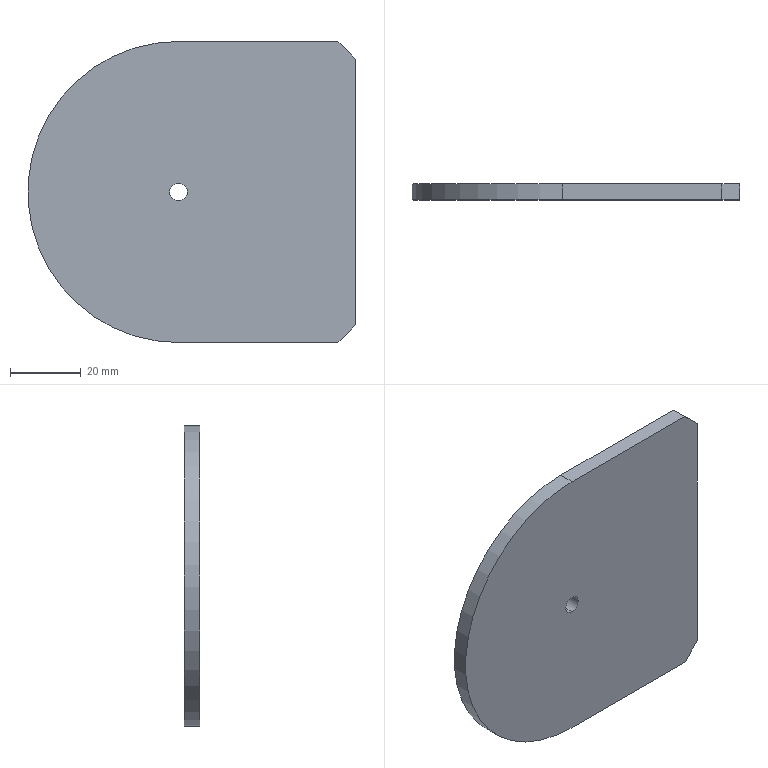Part | SolidWorks | features FlatPattern 1, SMBaseFlange 1, SheetMetal 1 | 1 solid | 10 faces | box 92.5 x 4.5 x 85 mm | volume 31692 mm3 | plane 7 | cylinder 3 | commonest cylinder face diameters 5 x2 85 x1
STEP:
#1=CARTESIAN_POINT('',(0.,-4.5,-2.5));
#2=VERTEX_POINT('',#1);
#3=CARTESIAN_POINT('',(0.,-4.5,2.5));
#4=VERTEX_POINT('',#3);
#5=CARTESIAN_POINT('',(0.,-4.5,0.));
#6=DIRECTION('',(0.,1.,0.));
#7=DIRECTION('',(0.,0.,1.));
#8=AXIS2_PLACEMENT_3D('',#5,#6,#7);
#9=CIRCLE('',#8,2.5);
#10=EDGE_CURVE('',#2,#4,#9,.T.);
#11=ORIENTED_EDGE('',*,*,#10,.F.);
#12=CARTESIAN_POINT('',(0.,0.,-2.5));
#13=VERTEX_POINT('',#12);
#14=CARTESIAN_POINT('',(0.,-4.5,-2.5));
#15=DIRECTION('',(0.,1.,0.));
#16=VECTOR('',#15,1000.);
#17=LINE('',#14,#16);
#18=EDGE_CURVE('',#2,#13,#17,.T.);
#19=ORIENTED_EDGE('',*,*,#18,.T.);
#20=CARTESIAN_POINT('',(0.,0.,2.5));
#21=VERTEX_POINT('',#20);
#22=CARTESIAN_POINT('',(0.,0.,0.));
#23=DIRECTION('',(0.,1.,0.));
#24=DIRECTION('',(0.,0.,1.));
#25=AXIS2_PLACEMENT_3D('',#22,#23,#24);
#26=CIRCLE('',#25,2.5);
#27=EDGE_CURVE('',#13,#21,#26,.T.);
#28=ORIENTED_EDGE('',*,*,#27,.T.);
#29=CARTESIAN_POINT('',(0.,-4.5,2.5));
#30=DIRECTION('',(0.,1.,0.));
#31=VECTOR('',#30,1000.);
#32=LINE('',#29,#31);
#33=EDGE_CURVE('',#4,#21,#32,.T.);
#34=ORIENTED_EDGE('',*,*,#33,.F.);
#35=EDGE_LOOP('',(#11,#19,#28,#34));
#36=FACE_OUTER_BOUND('',#35,.T.);
#37=CARTESIAN_POINT('',(0.,-4.5,0.));
#38=DIRECTION('',(0.,1.,0.));
#39=DIRECTION('',(0.,0.,1.));
#40=AXIS2_PLACEMENT_3D('',#37,#38,#39);
#41=CYLINDRICAL_SURFACE('',#40,2.5);
#42=ADVANCED_FACE('',(#36),#41,.F.);
#43=CARTESIAN_POINT('',(45.,0.,42.5));
#44=VERTEX_POINT('',#43);
#45=CARTESIAN_POINT('',(50.,0.,37.5));
#46=VERTEX_POINT('',#45);
#47=CARTESIAN_POINT('',(45.,0.,42.5));
#48=DIRECTION('',(0.7071,0.,-0.7071));
#49=VECTOR('',#48,1000.);
#50=LINE('',#47,#49);
#51=EDGE_CURVE('',#44,#46,#50,.T.);
#52=ORIENTED_EDGE('',*,*,#51,.F.);
#53=CARTESIAN_POINT('',(45.,-4.5,42.5));
#54=VERTEX_POINT('',#53);
#55=CARTESIAN_POINT('',(45.,-4.5,42.5));
#56=DIRECTION('',(0.,1.,0.));
#57=VECTOR('',#56,1000.);
#58=LINE('',#55,#57);
#59=EDGE_CURVE('',#54,#44,#58,.T.);
#60=ORIENTED_EDGE('',*,*,#59,.F.);
#61=CARTESIAN_POINT('',(50.,-4.5,37.5));
#62=VERTEX_POINT('',#61);
#63=CARTESIAN_POINT('',(45.,-4.5,42.5));
#64=DIRECTION('',(0.7071,0.,-0.7071));
#65=VECTOR('',#64,1000.);
#66=LINE('',#63,#65);
#67=EDGE_CURVE('',#54,#62,#66,.T.);
#68=ORIENTED_EDGE('',*,*,#67,.T.);
#69=CARTESIAN_POINT('',(50.,-4.5,37.5));
#70=DIRECTION('',(0.,1.,0.));
#71=VECTOR('',#70,1000.);
#72=LINE('',#69,#71);
#73=EDGE_CURVE('',#62,#46,#72,.T.);
#74=ORIENTED_EDGE('',*,*,#73,.T.);
#75=EDGE_LOOP('',(#52,#60,#68,#74));
#76=FACE_OUTER_BOUND('',#75,.T.);
#77=CARTESIAN_POINT('',(45.,-4.5,42.5));
#78=DIRECTION('',(0.7071,0.,0.7071));
#79=DIRECTION('',(0.7071,0.,-0.7071));
#80=AXIS2_PLACEMENT_3D('',#77,#78,#79);
#81=PLANE('',#80);
#82=ADVANCED_FACE('',(#76),#81,.T.);
#83=CARTESIAN_POINT('',(0.,0.,42.5));
#84=VERTEX_POINT('',#83);
#85=CARTESIAN_POINT('',(0.,0.,42.5));
#86=DIRECTION('',(1.,0.,0.));
#87=VECTOR('',#86,1000.);
#88=LINE('',#85,#87);
#89=EDGE_CURVE('',#84,#44,#88,.T.);
#90=ORIENTED_EDGE('',*,*,#89,.F.);
#91=CARTESIAN_POINT('',(0.,-4.5,42.5));
#92=VERTEX_POINT('',#91);
#93=CARTESIAN_POINT('',(0.,-4.5,42.5));
#94=DIRECTION('',(0.,1.,0.));
#95=VECTOR('',#94,1000.);
#96=LINE('',#93,#95);
#97=EDGE_CURVE('',#92,#84,#96,.T.);
#98=ORIENTED_EDGE('',*,*,#97,.F.);
#99=CARTESIAN_POINT('',(0.,-4.5,42.5));
#100=DIRECTION('',(1.,0.,0.));
#101=VECTOR('',#100,1000.);
#102=LINE('',#99,#101);
#103=EDGE_CURVE('',#92,#54,#102,.T.);
#104=ORIENTED_EDGE('',*,*,#103,.T.);
#105=ORIENTED_EDGE('',*,*,#59,.T.);
#106=EDGE_LOOP('',(#90,#98,#104,#105));
#107=FACE_OUTER_BOUND('',#106,.T.);
#108=CARTESIAN_POINT('',(0.,-4.5,42.5));
#109=DIRECTION('',(0.,0.,1.));
#110=DIRECTION('',(1.,0.,0.));
#111=AXIS2_PLACEMENT_3D('',#108,#109,#110);
#112=PLANE('',#111);
#113=ADVANCED_FACE('',(#107),#112,.T.);
#114=CARTESIAN_POINT('',(0.,0.,-42.5));
#115=VERTEX_POINT('',#114);
#116=CARTESIAN_POINT('',(0.,0.,0.));
#117=DIRECTION('',(0.,1.,0.));
#118=DIRECTION('',(0.,0.,1.));
#119=AXIS2_PLACEMENT_3D('',#116,#117,#118);
#120=CIRCLE('',#119,42.5);
#121=EDGE_CURVE('',#115,#84,#120,.T.);
#122=ORIENTED_EDGE('',*,*,#121,.F.);
#123=CARTESIAN_POINT('',(0.,-4.5,-42.5));
#124=VERTEX_POINT('',#123);
#125=CARTESIAN_POINT('',(0.,-4.5,-42.5));
#126=DIRECTION('',(0.,1.,0.));
#127=VECTOR('',#126,1000.);
#128=LINE('',#125,#127);
#129=EDGE_CURVE('',#124,#115,#128,.T.);
#130=ORIENTED_EDGE('',*,*,#129,.F.);
#131=CARTESIAN_POINT('',(0.,-4.5,0.));
#132=DIRECTION('',(0.,1.,0.));
#133=DIRECTION('',(0.,0.,1.));
#134=AXIS2_PLACEMENT_3D('',#131,#132,#133);
#135=CIRCLE('',#134,42.5);
#136=EDGE_CURVE('',#124,#92,#135,.T.);
#137=ORIENTED_EDGE('',*,*,#136,.T.);
#138=ORIENTED_EDGE('',*,*,#97,.T.);
#139=EDGE_LOOP('',(#122,#130,#137,#138));
#140=FACE_OUTER_BOUND('',#139,.T.);
#141=CARTESIAN_POINT('',(0.,-4.5,0.));
#142=DIRECTION('',(0.,1.,0.));
#143=DIRECTION('',(0.,0.,1.));
#144=AXIS2_PLACEMENT_3D('',#141,#142,#143);
#145=CYLINDRICAL_SURFACE('',#144,42.5);
#146=ADVANCED_FACE('',(#140),#145,.T.);
#147=CARTESIAN_POINT('',(45.,0.,-42.5));
#148=VERTEX_POINT('',#147);
#149=CARTESIAN_POINT('',(45.,0.,-42.5));
#150=DIRECTION('',(-1.,0.,0.));
#151=VECTOR('',#150,1000.);
#152=LINE('',#149,#151);
#153=EDGE_CURVE('',#148,#115,#152,.T.);
#154=ORIENTED_EDGE('',*,*,#153,.F.);
#155=CARTESIAN_POINT('',(45.,-4.5,-42.5));
#156=VERTEX_POINT('',#155);
#157=CARTESIAN_POINT('',(45.,-4.5,-42.5));
#158=DIRECTION('',(0.,1.,0.));
#159=VECTOR('',#158,1000.);
#160=LINE('',#157,#159);
#161=EDGE_CURVE('',#156,#148,#160,.T.);
#162=ORIENTED_EDGE('',*,*,#161,.F.);
#163=CARTESIAN_POINT('',(45.,-4.5,-42.5));
#164=DIRECTION('',(-1.,0.,0.));
#165=VECTOR('',#164,1000.);
#166=LINE('',#163,#165);
#167=EDGE_CURVE('',#156,#124,#166,.T.);
#168=ORIENTED_EDGE('',*,*,#167,.T.);
#169=ORIENTED_EDGE('',*,*,#129,.T.);
#170=EDGE_LOOP('',(#154,#162,#168,#169));
#171=FACE_OUTER_BOUND('',#170,.T.);
#172=CARTESIAN_POINT('',(45.,-4.5,-42.5));
#173=DIRECTION('',(0.,0.,-1.));
#174=DIRECTION('',(-1.,0.,0.));
#175=AXIS2_PLACEMENT_3D('',#172,#173,#174);
#176=PLANE('',#175);
#177=ADVANCED_FACE('',(#171),#176,.T.);
#178=CARTESIAN_POINT('',(50.,0.,-37.5));
#179=VERTEX_POINT('',#178);
#180=CARTESIAN_POINT('',(50.,0.,-37.5));
#181=DIRECTION('',(-0.7071,0.,-0.7071));
#182=VECTOR('',#181,1000.);
#183=LINE('',#180,#182);
#184=EDGE_CURVE('',#179,#148,#183,.T.);
#185=ORIENTED_EDGE('',*,*,#184,.F.);
#186=CARTESIAN_POINT('',(50.,-4.5,-37.5));
#187=VERTEX_POINT('',#186);
#188=CARTESIAN_POINT('',(50.,-4.5,-37.5));
#189=DIRECTION('',(0.,1.,0.));
#190=VECTOR('',#189,1000.);
#191=LINE('',#188,#190);
#192=EDGE_CURVE('',#187,#179,#191,.T.);
#193=ORIENTED_EDGE('',*,*,#192,.F.);
#194=CARTESIAN_POINT('',(50.,-4.5,-37.5));
#195=DIRECTION('',(-0.7071,0.,-0.7071));
#196=VECTOR('',#195,1000.);
#197=LINE('',#194,#196);
#198=EDGE_CURVE('',#187,#156,#197,.T.);
#199=ORIENTED_EDGE('',*,*,#198,.T.);
#200=ORIENTED_EDGE('',*,*,#161,.T.);
#201=EDGE_LOOP('',(#185,#193,#199,#200));
#202=FACE_OUTER_BOUND('',#201,.T.);
#203=CARTESIAN_POINT('',(50.,-4.5,-37.5));
#204=DIRECTION('',(0.7071,0.,-0.7071));
#205=DIRECTION('',(-0.7071,0.,-0.7071));
#206=AXIS2_PLACEMENT_3D('',#203,#204,#205);
#207=PLANE('',#206);
#208=ADVANCED_FACE('',(#202),#207,.T.);
#209=CARTESIAN_POINT('',(50.,0.,37.5));
#210=DIRECTION('',(0.,0.,-1.));
#211=VECTOR('',#210,1000.);
#212=LINE('',#209,#211);
#213=EDGE_CURVE('',#46,#179,#212,.T.);
#214=ORIENTED_EDGE('',*,*,#213,.F.);
#215=ORIENTED_EDGE('',*,*,#73,.F.);
#216=CARTESIAN_POINT('',(50.,-4.5,37.5));
#217=DIRECTION('',(0.,0.,-1.));
#218=VECTOR('',#217,1000.);
#219=LINE('',#216,#218);
#220=EDGE_CURVE('',#62,#187,#219,.T.);
#221=ORIENTED_EDGE('',*,*,#220,.T.);
#222=ORIENTED_EDGE('',*,*,#192,.T.);
#223=EDGE_LOOP('',(#214,#215,#221,#222));
#224=FACE_OUTER_BOUND('',#223,.T.);
#225=CARTESIAN_POINT('',(50.,-4.5,37.5));
#226=DIRECTION('',(1.,0.,0.));
#227=DIRECTION('',(0.,0.,-1.));
#228=AXIS2_PLACEMENT_3D('',#225,#226,#227);
#229=PLANE('',#228);
#230=ADVANCED_FACE('',(#224),#229,.T.);
#231=CARTESIAN_POINT('',(0.,-4.5,0.));
#232=DIRECTION('',(0.,1.,0.));
#233=DIRECTION('',(0.,0.,1.));
#234=AXIS2_PLACEMENT_3D('',#231,#232,#233);
#235=CIRCLE('',#234,2.5);
#236=EDGE_CURVE('',#4,#2,#235,.T.);
#237=ORIENTED_EDGE('',*,*,#236,.T.);
#238=ORIENTED_EDGE('',*,*,#10,.T.);
#239=EDGE_LOOP('',(#237,#238));
#240=FACE_BOUND('',#239,.T.);
#241=ORIENTED_EDGE('',*,*,#67,.F.);
#242=ORIENTED_EDGE('',*,*,#103,.F.);
#243=ORIENTED_EDGE('',*,*,#136,.F.);
#244=ORIENTED_EDGE('',*,*,#167,.F.);
#245=ORIENTED_EDGE('',*,*,#198,.F.);
#246=ORIENTED_EDGE('',*,*,#220,.F.);
#247=EDGE_LOOP('',(#241,#242,#243,#244,#245,#246));
#248=FACE_OUTER_BOUND('',#247,.T.);
#249=CARTESIAN_POINT('',(0.,-4.5,0.));
#250=DIRECTION('',(0.,1.,0.));
#251=DIRECTION('',(0.,0.,1.));
#252=AXIS2_PLACEMENT_3D('',#249,#250,#251);
#253=PLANE('',#252);
#254=ADVANCED_FACE('',(#240,#248),#253,.F.);
#255=CARTESIAN_POINT('',(0.,0.,0.));
#256=DIRECTION('',(0.,1.,0.));
#257=DIRECTION('',(0.,0.,1.));
#258=AXIS2_PLACEMENT_3D('',#255,#256,#257);
#259=CIRCLE('',#258,2.5);
#260=EDGE_CURVE('',#21,#13,#259,.T.);
#261=ORIENTED_EDGE('',*,*,#260,.F.);
#262=ORIENTED_EDGE('',*,*,#27,.F.);
#263=EDGE_LOOP('',(#261,#262));
#264=FACE_BOUND('',#263,.T.);
#265=ORIENTED_EDGE('',*,*,#51,.T.);
#266=ORIENTED_EDGE('',*,*,#213,.T.);
#267=ORIENTED_EDGE('',*,*,#184,.T.);
#268=ORIENTED_EDGE('',*,*,#153,.T.);
#269=ORIENTED_EDGE('',*,*,#121,.T.);
#270=ORIENTED_EDGE('',*,*,#89,.T.);
#271=EDGE_LOOP('',(#265,#266,#267,#268,#269,#270));
#272=FACE_OUTER_BOUND('',#271,.T.);
#273=CARTESIAN_POINT('',(0.,0.,0.));
#274=DIRECTION('',(0.,1.,0.));
#275=DIRECTION('',(0.,0.,1.));
#276=AXIS2_PLACEMENT_3D('',#273,#274,#275);
#277=PLANE('',#276);
#278=ADVANCED_FACE('',(#264,#272),#277,.T.);
#279=ORIENTED_EDGE('',*,*,#18,.F.);
#280=ORIENTED_EDGE('',*,*,#236,.F.);
#281=ORIENTED_EDGE('',*,*,#33,.T.);
#282=ORIENTED_EDGE('',*,*,#260,.T.);
#283=EDGE_LOOP('',(#279,#280,#281,#282));
#284=FACE_OUTER_BOUND('',#283,.T.);
#285=CARTESIAN_POINT('',(0.,-4.5,0.));
#286=DIRECTION('',(0.,1.,0.));
#287=DIRECTION('',(0.,0.,1.));
#288=AXIS2_PLACEMENT_3D('',#285,#286,#287);
#289=CYLINDRICAL_SURFACE('',#288,2.5);
#290=ADVANCED_FACE('',(#284),#289,.F.);
#291=CLOSED_SHELL('',(#42,#82,#113,#146,#177,#208,#230,#254,#278,#290));
#292=MANIFOLD_SOLID_BREP('',#291);
#293=CARTESIAN_POINT('',(0.,0.,0.));
#294=DIRECTION('',(0.,0.,1.));
#295=DIRECTION('',(1.,0.,0.));
#296=AXIS2_PLACEMENT_3D('',#293,#294,#295);
#297=(LENGTH_UNIT()NAMED_UNIT(*)SI_UNIT(.MILLI.,.METRE.));
#298=UNCERTAINTY_MEASURE_WITH_UNIT(LENGTH_MEASURE(0.00001),#297,'','');
#299=(NAMED_UNIT(*)PLANE_ANGLE_UNIT()SI_UNIT($,.RADIAN.));
#300=(NAMED_UNIT(*)SI_UNIT($,.STERADIAN.)SOLID_ANGLE_UNIT());
#301=(GEOMETRIC_REPRESENTATION_CONTEXT(3)GLOBAL_UNCERTAINTY_ASSIGNED_CONTEXT((#298))GLOBAL_UNIT_ASSIGNED_CONTEXT((#297,#299,#300))REPRESENTATION_CONTEXT('',''));
#302=ADVANCED_BREP_SHAPE_REPRESENTATION('',(#292,#296),#301);